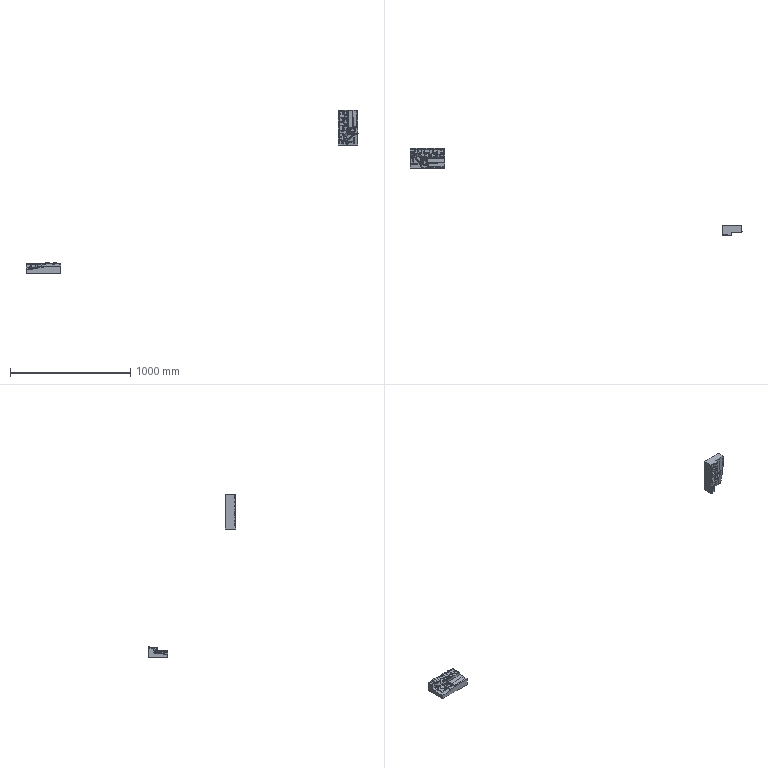NC program | NX | posted with a generic post | part box 2756 x 729.572 x 1353 mm
Lines 43585 to 44366 of 54396:
(ZLEVEL_PROFILE_3 , TOOL : D12)
N87150 M6
N87152 G54
N87154 G17 G0 G90 X-15.26 Y-84.156 B0. C0. S3000 M3
N87156 G43 Z97. H0
N87158 Z82.254
N87160 G94 G1 X-2.438 Y-83.975 Z81.918 F2500.
N87162 X0. Y-83.973 Z81.854
N87164 X-2.438 Y-83.975
N87166 X-31.79 Y-84.389
N87168 X-41.451 Y-84.428
N87170 X-43.147 Y-84.322
N87172 G2 X-50.227 Y-77.434 R7.65
N87174 G1 X-51.514 Y-77.439 Z81.655
N87176 G3 X-47.378 Y-83.482 R6.752
N87178 X-41.451 Y-84.694 R15.56
N87180 G1 X0. Y-84.333
N87182 Z84.655
N87184 G0 Z97.
N87186 X-76.288 Y-83.954
N87188 Z82.254
N87190 G1 X-72.831 Y-84.154 Z82.163
N87192 X-71.135 Y-84.11 Z82.119
N87194 X-70.497 Y-84.08 Z82.102
N87196 X-68.796 Y-83.61 Z82.056
N87198 X-67.273 Y-82.718 Z82.01
N87200 X-66.03 Y-81.466 Z81.964
N87202 X-65.15 Y-79.936 Z81.917
N87204 X-64.693 Y-78.231 Z81.871
N87206 X-64.668 Y-77.593 Z81.854
N87208 G2 X-71.135 Y-84.11 R6.785
N87210 G1 X-72.831 Y-84.154
N87212 X-83.009 Y-83.563
N87214 X-83.167 Y-83.542
N87216 X-87.688 Y-80.237
N87218 Z84.854
N87220 G0 Z97.
N87222 X-86.71 Y-84.276
N87224 Z82.054
N87226 G1 X-90.277 Y-84.161 Z81.961
N87228 X-95.479 Y-83.84 Z81.825
N87230 X-96.889 Y-83.466 Z81.786
N87232 X-98.189 Y-82.805 Z81.748
N87234 X-99.324 Y-81.888 Z81.71
N87236 X-100.241 Y-80.755 Z81.672
N87238 X-100.541 Y-80.183 Z81.655
N87240 G3 X-94.835 Y-83.88 R6.922
N87242 X-74.528 Y-84.537 R347.568
N87244 G1 X-73.463 Y-84.597
N87246 G3 X-68.845 Y-84.09 R14.083
N87248 X-63.737 Y-77.565 R7.018
N87250 G1 X-63.393 Y-77.56 Z81.555
N87252 X-63.108 Y-77.556 Z81.455
N87254 G2 X-66.891 Y-83.651 R7.004
N87256 X-71.649 Y-84.818 R10.426
N87258 X-104.334 Y-84.066 R619.573
N87260 X-111.303 Y-79.673 R8.39
N87262 G1 Z84.455
N87264 G0 Z97.
N87266 X-15.26 Y-84.692
N87268 Z81.855
N87270 G1 X-2.438 Y-84.565 Z81.519
N87272 X0. Y-84.592 Z81.455
N87274 X-2.438 Y-84.565
N87276 X-18.552 Y-84.725
N87278 X-22.793 Y-84.765
N87280 X-41.451 Y-84.881
N87282 G2 X-48.498 Y-83.558 R19.928
N87284 X-52.802 Y-77.444 R6.709
N87286 G1 X-54.089 Y-77.449 Z81.256
N87288 G3 X-49.43 Y-83.717 R6.783
N87290 X-41.451 Y-85.03 R26.196
N87292 G1 X-4.134 Y-84.771
N87294 X0.003 Y-84.763
N87296 Z84.256
N87298 G0 Z97.
N87300 X-73.803 Y-85.035
N87302 Z81.655
N87304 G1 X-71.983 Y-85.034 Z81.608
N87306 X-71.109 Y-85.039 Z81.585
N87308 X-69.38 Y-84.808 Z81.539
N87310 X-67.698 Y-84.345 Z81.493
N87312 X-66.895 Y-83.999 Z81.47
N87314 X-66.291 Y-83.731 Z81.453
N87316 X-64.897 Y-82.723 Z81.408
N87318 X-63.778 Y-81.416 Z81.363
N87320 X-62.997 Y-79.883 Z81.318
N87322 X-62.596 Y-78.21 Z81.273
N87324 X-62.579 Y-77.55 Z81.256
N87326 G2 X-66.895 Y-83.999 R7.261
N87328 X-71.983 Y-85.034 R12.732
N87330 X-109.155 Y-84.389 R1066.044
N87332 G1 X-115.237 Y-83.793
N87334 X-116.299 Y-83.542
N87336 X-116.933 Y-83.253
N87338 X-120.751 Y-78.147
N87340 Z84.256
N87342 G0 Z97.
N87344 X-115.867 Y-84.489
N87346 Z81.456
N87348 G1 X-119.405 Y-84.298 Z81.363
N87350 X-122.87 Y-83.978 Z81.272
N87352 X-123.501 Y-83.932 Z81.255
N87354 X-125.167 Y-83.42 Z81.21
N87356 X-126.644 Y-82.494 Z81.164
N87358 X-127.831 Y-81.217 Z81.118
N87360 X-128.646 Y-79.676 Z81.073
N87362 X-128.81 Y-79.066 Z81.056
N87364 G3 X-122.87 Y-83.978 R6.646
N87366 X-107.604 Y-84.805 R201.793
N87368 X-71.983 Y-85.161 R1612.787
N87370 G1 X-71.135 Y-85.134
N87372 G3 X-66.895 Y-84.243 R11.864
N87374 X-62.162 Y-77.545 R7.318
N87376 G1 Z84.056
N87378 G0 Z97.
N87380 X-15.258 Y-84.985
N87382 Z81.456
N87384 G1 X-5.828 Y-84.9 Z81.209
N87386 X0.003 Y-84.891 Z81.056
N87388 G3 X-11.659 Y-84.952 R1562.88
N87390 G2 X-41.451 Y-85.119 R4404.057
N87392 X-50.375 Y-83.867 R32.265
N87394 X-55.377 Y-77.455 R6.912
N87396 G1 X-56.665 Y-77.46 Z80.856
N87398 G3 X-53.377 Y-83.029 R6.44
N87400 X-49.749 Y-84.374 R12.414
N87402 X-41.309 Y-85.197 R41.905
N87404 G1 X-21.096 Y-85.111
N87406 G2 X0. Y-85.003 R1960.321
N87408 G1 Z83.856
N87410 G0 Z97.
N87412 X-72.868 Y-85.26
N87414 Z81.256
N87416 G1 X-71.135 Y-85.251 Z81.211
N87418 X-70.264 Y-85.238 Z81.188
N87420 X-68.524 Y-84.967 Z81.142
N87422 X-66.837 Y-84.458 Z81.096
N87424 X-66.047 Y-84.093 Z81.073
N87426 X-65.441 Y-83.811 Z81.055
N87428 X-64.055 Y-82.773 Z81.01
N87430 X-62.945 Y-81.444 Z80.965
N87432 X-62.171 Y-79.895 Z80.919
N87434 X-61.775 Y-78.21 Z80.874
N87436 X-61.758 Y-77.542 Z80.856
N87438 G2 X-66.047 Y-84.093 R7.435
N87440 X-71.135 Y-85.251 R12.626
N87442 X-117.782 Y-84.813 R1613.418
N87444 X-130.503 Y-83.973 R149.134
N87446 X-135.944 Y-80.062 R6.777
N87448 G1 X-136.372 Y-80.074 Z80.845
N87450 X-136.795 Y-80.083 Z80.833
N87452 X-137.219 Y-80.093 Z80.821
N87454 X-137.638 Y-80.1 Z80.809
N87456 X-138.035 Y-80.097 Z80.798
N87458 X-138.43 Y-80.093 Z80.786
N87460 X-138.826 Y-80.09 Z80.774
N87462 X-139.222 Y-80.086 Z80.762
N87464 X-139.618 Y-80.083 Z80.751
N87466 X-140.014 Y-80.08 Z80.739
N87468 X-140.409 Y-80.076 Z80.727
N87470 X-140.805 Y-80.073 Z80.715
N87472 X-141.2 Y-80.069 Z80.704
N87474 X-141.595 Y-80.065 Z80.692
N87476 X-141.991 Y-80.062 Z80.68
N87478 X-142.385 Y-80.058 Z80.669
N87480 X-142.779 Y-80.054 Z80.657
N87482 G3 X-137.418 Y-83.994 R6.767
N87484 X-125.542 Y-84.85 R124.376
N87486 X-71.135 Y-85.333 R1794.109
N87488 X-66.047 Y-84.307 R13.761
N87490 X-61.435 Y-77.539 R7.498
N87492 G1 Z83.657
N87494 G0 Z97.
N87496 X-15.255 Y-85.116
N87498 Z81.056
N87500 G1 X-14.786 Y-85.112 Z81.044
N87502 X0.006 Y-85.074 Z80.657
N87504 G3 X-29.578 Y-85.221 R6272.571
N87506 G1 X-41.451 Y-85.26
N87508 X-42.299 Y-85.272
N87510 G2 X-51.075 Y-84.389 R54.431
N87512 X-55.736 Y-82.252 R9.873
N87514 X-57.952 Y-77.465 R6.131
N87516 G1 X-59.24 Y-77.47 Z80.457
N87518 G3 X-57.002 Y-82.275 R6.156
N87520 X-52.529 Y-84.363 R9.858
N87522 X-42.235 Y-85.297 R55.422
N87524 G1 X-39.755 Y-85.29
N87526 X-16.856 Y-85.187
N87528 X-5.041 Y-85.125
N87530 G2 X-0.004 Y-85.131 R401.668
N87532 G1 Z83.457
N87534 G0 Z97.
N87536 X-72.13 Y-85.434
N87538 Z80.857
N87540 G1 X-72.02 Y-85.436 Z80.854
N87542 X-71.095 Y-85.41 Z80.83
N87544 X-69.439 Y-85.285 Z80.786
N87546 X-68.636 Y-85.227 Z80.765
N87548 X-67.248 Y-84.926 Z80.728
N87550 X-65.91 Y-84.445 Z80.691
N87552 X-65.198 Y-84.07 Z80.67
N87554 X-64.601 Y-83.767 Z80.652
N87556 X-63.276 Y-82.712 Z80.608
N87558 X-62.222 Y-81.387 Z80.563
N87560 X-61.492 Y-79.859 Z80.519
N87562 X-61.124 Y-78.207 Z80.475
N87564 X-61.113 Y-77.537 Z80.457
N87566 G2 X-65.198 Y-84.07 R7.468
N87568 X-69.439 Y-85.285 R10.776
N87570 X-73.68 Y-85.407 R45.93
N87572 G1 X-74.528 Y-85.392
N87574 G2 X-117.782 Y-85.229 R2539.324
N87576 X-142.923 Y-84.276 R450.056
N87578 X-149.269 Y-80.042 R7.642
N87580 G1 X-149.678 Y-80.041 Z80.444
N87582 X-150.085 Y-80.038 Z80.431
N87584 X-150.492 Y-80.036 Z80.417
N87586 X-150.899 Y-80.034 Z80.404
N87588 X-151.306 Y-80.032 Z80.391
N87590 X-151.713 Y-80.029 Z80.377
N87592 X-152.12 Y-80.027 Z80.364
N87594 X-152.528 Y-80.026 Z80.351
N87596 X-152.933 Y-80.023 Z80.337
N87598 X-153.34 Y-80.02 Z80.324
N87600 X-153.747 Y-80.018 Z80.311
N87602 X-154.154 Y-80.016 Z80.297
N87604 X-154.561 Y-80.014 Z80.284
N87606 X-154.968 Y-80.011 Z80.271
N87608 X-155.375 Y-80.009 Z80.258
N87610 G3 X-150.241 Y-84.012 R6.619
N87612 G1 X-149.162 Y-84.173
N87614 X-141.529 Y-84.814
N87616 G3 X-111.845 Y-85.42 R967.084
N87618 X-71.135 Y-85.414 R4122.292
N87620 G1 X-70.287 Y-85.401
N87622 G3 X-66.047 Y-84.618 R12.922
N87624 X-60.811 Y-77.534 R7.695
N87626 G1 Z83.258
N87628 G0 Z97.
N87630 X-15.266 Y-85.208
N87632 Z80.657
N87634 G1 X-3.286 Y-85.153 Z80.343
N87636 X-0.005 Y-85.158 Z80.258
N87638 X-3.286 Y-85.153
N87640 X-16.856 Y-85.215
N87642 X-42.299 Y-85.323
N87644 G2 X-51.295 Y-84.803 R74.498
N87646 X-56.208 Y-83.598 R20.754
N87648 X-60.527 Y-77.476 R6.696
N87650 G1 Z83.258
N87652 G0 Z97.
N87654 X-147.529 Y-84.844
N87656 Z80.458
N87658 G1 X-148.314 Y-84.813 Z80.437
N87660 X-150.016 Y-84.761 Z80.392
N87662 X-154.043 Y-84.328 Z80.286
N87664 X-156.381 Y-83.891 Z80.224
N87666 X-158.123 Y-83.159 Z80.175
N87668 X-159.631 Y-82.02 Z80.125
N87670 X-160.812 Y-80.545 Z80.076
N87672 X-161.112 Y-79.941 Z80.058
N87674 G3 X-155.717 Y-84.015 R7.578
N87676 X-148.314 Y-84.813 R48.317
N87678 X-121.174 Y-85.447 R801.832
N87680 X-70.287 Y-85.428 R4192.566
N87682 X-66.047 Y-84.761 R13.62
N87684 X-61.107 Y-80.35 R8.22
N87686 X-57.081 Y-83.781 R7.132
N87688 X-52.477 Y-84.819 R22.701
N87690 X-43.996 Y-85.33 R75.99
N87692 G1 X-4.982 Y-85.166
N87694 X0.001 Y-85.165
N87696 Z79.858
N87698 X-4.982 Y-85.166
N87700 X-44.844 Y-85.333
N87702 X-46.656 Y-85.317
N87704 G2 X-56.513 Y-84.355 R55.858
N87706 X-61.527 Y-81.644 R9.356
N87708 X-66.048 Y-84.871 R8.866
N87710 X-69.704 Y-85.437 R12.577
N87712 X-112.693 Y-85.549 R6359.498
N87714 X-143.225 Y-85.246 R1397.155
N87716 G1 X-143.737 Y-85.236
N87718 X-151.706 Y-84.939
N87720 X-152.554 Y-84.891
N87722 G2 X-162.732 Y-82.614 R30.47
N87724 X-167.024 Y-78.15 R7.436
N87726 G1 X-167.392 Y-77.962 Z79.847
N87728 X-167.746 Y-77.768 Z79.835
N87730 X-168.1 Y-77.575 Z79.823
N87732 X-168.454 Y-77.381 Z79.811
N87734 X-168.781 Y-77.18 Z79.8
N87736 X-169.124 Y-76.983 Z79.788
N87738 X-169.513 Y-76.799 Z79.776
N87740 X-169.864 Y-76.604 Z79.764
N87742 X-170.215 Y-76.41 Z79.753
N87744 X-170.564 Y-76.215 Z79.741
N87746 X-170.917 Y-76.02 Z79.729
N87748 X-171.259 Y-75.824 Z79.717
N87750 X-171.59 Y-75.625 Z79.706
N87752 X-171.954 Y-75.433 Z79.694
N87754 X-172.298 Y-75.237 Z79.682
N87756 X-172.641 Y-75.041 Z79.67
N87758 X-172.981 Y-74.845 Z79.659
N87760 G3 X-168.85 Y-80.672 R8.016
N87762 X-151.706 Y-85.203 R38.229
N87764 X-126.6 Y-85.575 R1114.804
N87766 X-103.563 Y-85.571 R3081.8
N87768 G1 X-69.439 Y-85.437
N87770 G3 X-66.895 Y-85.164 R12.488
N87772 X-61.928 Y-82.512 R9.408
N87774 X-56.945 Y-84.53 R12.152
N87776 X-46.54 Y-85.34 R62.082
N87778 G1 X-4.982 Y-85.166
N87780 X0.001 Y-85.165
N87782 Z79.459
N87784 X-4.982 Y-85.166
N87786 X-48.236 Y-85.34
N87788 G2 X-58.362 Y-84.501 R58.672
N87790 X-62.256 Y-83.125 R12.186
N87792 X-68.591 Y-85.419 R10.432
N87794 G1 X-69.439 Y-85.437
N87796 X-114.389 Y-85.626
N87798 X-126.067 Y-85.621
N87800 G2 X-151.818 Y-85.37 R1382.193
N87802 X-175.375 Y-77.615 R42.102
N87804 X-178.764 Y-72.06 R8.26
N87806 G1 X-179.116 Y-71.85 Z79.447
N87808 X-179.459 Y-71.639 Z79.436
N87810 X-179.803 Y-71.428 Z79.424
N87812 X-180.146 Y-71.217 Z79.412
N87814 X-180.49 Y-71.006 Z79.4
N87816 X-180.833 Y-70.795 Z79.389
N87818 X-181.177 Y-70.584 Z79.377
N87820 X-181.521 Y-70.373 Z79.365
N87822 X-181.864 Y-70.162 Z79.353
N87824 X-182.208 Y-69.951 Z79.342
N87826 X-182.551 Y-69.74 Z79.33
N87828 X-182.895 Y-69.529 Z79.318
N87830 X-183.239 Y-69.318 Z79.306
N87832 X-183.582 Y-69.107 Z79.295
N87834 X-183.926 Y-68.896 Z79.283
N87836 X-184.269 Y-68.686 Z79.271
N87838 X-184.605 Y-68.47 Z79.259
N87840 X-182.089 Y-73.381
N87842 X-181.39 Y-74.122
N87844 G3 X-151.706 Y-85.521 R46.715
N87846 X-117.782 Y-85.642 R2121.63
N87848 G1 X-68.591 Y-85.432
N87850 G3 X-62.558 Y-83.66 R11.672
N87852 X-58.694 Y-84.674 R18.227
N87854 X-49.084 Y-85.35 R62.914
N87856 G1 X-4.982 Y-85.166
N87858 X0.001 Y-85.165
N87860 Z79.06
N87862 X-4.982 Y-85.166
N87864 X-49.932 Y-85.355
N87866 G2 X-59.262 Y-84.799 R69.021
N87868 X-62.788 Y-84.029 R20.683
N87870 X-68.591 Y-85.432 R12.548
N87872 G1 X-124.159 Y-85.669
N87874 G2 X-151.229 Y-85.628 R2342.368
N87876 X-161.035 Y-84.597 R50.724
N87878 X-188.175 Y-68.956 R52.233
N87880 G1 X-188.736 Y-68.3
N87882 X-190.408 Y-64.913
N87884 X-190.506 Y-64.151
N87886 X-190.84 Y-63.908 Z79.049
N87888 X-191.168 Y-63.665 Z79.038
N87890 X-191.496 Y-63.422 Z79.027
N87892 X-191.825 Y-63.178 Z79.015
N87894 X-192.153 Y-62.935 Z79.004
N87896 X-192.481 Y-62.692 Z78.993
N87898 X-192.809 Y-62.448 Z78.982
N87900 X-193.137 Y-62.205 Z78.971
N87902 X-193.465 Y-61.962 Z78.96
N87904 X-193.794 Y-61.718 Z78.949
N87906 X-194.122 Y-61.475 Z78.938
N87908 X-194.45 Y-61.231 Z78.927
N87910 X-194.778 Y-60.988 Z78.916
N87912 X-195.106 Y-60.745 Z78.905
N87914 X-195.434 Y-60.501 Z78.893
N87916 X-195.763 Y-60.258 Z78.882
N87918 X-196.091 Y-60.014 Z78.871
N87920 X-196.418 Y-59.771 Z78.86
N87922 G3 X-193.297 Y-65.246 R14.336
N87924 X-175.751 Y-79.308 R72.566
N87926 X-151.706 Y-85.699 R50.267
N87928 G1 X-133.896 Y-85.71
N87930 X-67.743 Y-85.421
N87932 G3 X-62.972 Y-84.359 R14.903
N87934 X-58.414 Y-85.053 R39.933
N87936 X-51.629 Y-85.361 R77.462
N87938 G1 X-4.982 Y-85.166
N87940 X0.001 Y-85.165
N87942 Z78.661
N87944 X-4.982 Y-85.166
N87946 X-53.13 Y-85.367
N87948 G2 X-63.037 Y-84.62 R62.606
N87950 G1 X-65.111 Y-85.11
N87952 G2 X-67.816 Y-85.431 R11.986
N87954 G1 X-143.225 Y-85.748
N87956 X-152.554 Y-85.725
N87958 X-154.251 Y-85.681
N87960 G2 X-176.616 Y-79.18 R51.501
N87962 X-189.023 Y-70.199 R66.39
N87964 X-200.313 Y-59.833 R117.66
N87966 G1 X-200.897 Y-59.055
N87968 X-202.324 Y-55.39
N87970 Z81.661
N87972 G0 Z97.
N87974 X-233.773 Y-47.613
N87976 Z81.056
N87978 G1 X-231.945 Y-47.26 Z81.008
N87980 X-230.581 Y-46.874 Z80.971
N87982 X-230.021 Y-46.662 Z80.955
N87984 X-228.743 Y-45.803 Z80.915
N87986 X-227.726 Y-44.645 Z80.874
N87988 X-227.038 Y-43.266 Z80.834
N87990 X-226.726 Y-41.758 Z80.793
N87992 X-226.808 Y-40.219 Z80.753
N87994 X-227.281 Y-38.753 Z80.713
N87996 X-228.113 Y-37.456 Z80.672
N87998 X-228.542 Y-37.039 Z80.657
N88000 G2 X-230.581 Y-46.874 R5.954
N88002 X-241.798 Y-48.07 R33.455
N88004 X-248.063 Y-40.695 R6.722
N88006 G1 X-248.442 Y-40.848 Z80.557
N88008 X-248.709 Y-41.008 Z80.457
N88010 G3 X-240.598 Y-48.951 R7.685
N88012 G2 X-223.856 Y-48.894 R159.009
N88014 G3 X-216.714 Y-43.031 R6.877
N88016 G1 X-216.347 Y-43.263 Z80.357
N88018 X-216.115 Y-43.472 Z80.258
N88020 G2 X-224.644 Y-49.614 R7.705
N88022 G1 X-225.492 Y-49.503
N88024 G3 X-240.758 Y-49.42 R118.273
N88026 G2 X-249.122 Y-41.068 R8.095
N88028 G1 X-249.3 Y-41.087 Z80.158
N88030 X-249.443 Y-41.102 Z80.058
N88032 G3 X-240.758 Y-49.793 R8.457
N88034 G1 X-232.277 Y-49.686
N88036 G2 X-224.644 Y-50.093 R55.651
N88038 G3 X-215.718 Y-43.609 R8.158
N88040 G1 X-215.556 Y-43.673 Z79.958
N88042 X-215.406 Y-43.732 Z79.858
N88044 G2 X-224.759 Y-50.443 R8.507
N88046 G3 X-232.277 Y-50.025 R57.669
N88048 G1 X-240.758 Y-50.114
N88050 G2 X-249.53 Y-42.898 R8.639
N88052 X-249.719 Y-41.125 R6.395
N88054 G1 X-249.836 Y-41.137 Z79.758
N88056 X-249.942 Y-41.148 Z79.659
N88058 G3 X-240.758 Y-50.368 R9.012
N88060 G1 X-232.277 Y-50.309
N88062 G2 X-224.85 Y-50.74 R55.695
N88064 G3 X-215.139 Y-43.751 R8.789
N88066 G1 X-215.024 Y-43.396 Z79.619
N88068 X-214.925 Y-43.036 Z79.579
N88070 X-214.833 Y-42.674 Z79.539
N88072 X-214.765 Y-42.31 Z79.499
N88074 X-214.719 Y-41.949 Z79.459
N88076 G2 X-224.974 Y-51.001 R9.063
N88078 G3 X-232.277 Y-50.564 R50.782
N88080 G1 X-240.758 Y-50.601
N88082 X-241.05 Y-50.597
N88084 G2 X-250.163 Y-41.182 R9.24
N88086 G1 X-250.272 Y-41.205 Z79.359
N88088 X-250.404 Y-41.232 Z79.259
N88090 G3 X-241.05 Y-50.799 R9.492
N88092 G1 X-240.758 Y-50.803
N88094 X-233.125 Y-50.769
N88096 G2 X-224.644 Y-51.255 R61.029
N88098 G3 X-217.859 Y-49.145 R9.075
N88100 X-214.493 Y-41.659 R8.833
N88102 G1 X-214.354 Y-41.666 Z79.16
N88104 X-214.211 Y-41.674 Z79.06
N88106 G2 X-216.736 Y-48.439 R8.621
N88108 G1 X-216.961 Y-48.662
N88110 G2 X-225.215 Y-51.412 R9.802
N88112 G3 X-230.581 Y-50.99 R44.959
N88114 G1 X-232.277 Y-50.965
N88116 X-240.758 Y-50.991
N88118 G2 X-247.543 Y-48.31 R9.389
N88120 X-250.661 Y-41.28 R9.289
N88122 G1 X-250.781 Y-41.303 Z78.96
N88124 X-250.922 Y-41.329 Z78.86
N88126 G3 X-247.543 Y-48.558 R9.162
N88128 X-241.182 Y-51.137 R9.711
N88130 G1 X-240.758 Y-51.148
N88132 X-233.125 Y-51.13
N88134 G2 X-225.009 Y-51.593 R62.326
N88136 G3 X-217.648 Y-49.57 R10.025
N88138 G1 X-217.011 Y-49.077
N88140 G3 X-213.915 Y-41.714 R8.498
N88142 G1 X-213.591 Y-41.769 Z78.661
N88144 G2 X-218.721 Y-50.519 R8.717
N88146 X-224.644 Y-51.811 R10.732
N88148 G3 X-230.648 Y-51.329 R52.182
N88150 G1 X-232.277 Y-51.293
N88152 X-240.758 Y-51.304
N88154 G2 X-246.695 Y-49.431 R9.989
N88156 X-250.718 Y-44.591 R10.694
N88158 X-251.278 Y-41.363 R9.119
N88160 G1 X-251.431 Y-41.377 Z78.561
N88162 X-251.639 Y-41.396 Z78.461
N88164 G3 X-250.717 Y-45.438 R7.355
N88166 X-245.847 Y-50.118 R11.606
N88168 X-240.758 Y-51.432 R9.828
N88170 G1 X-232.277 Y-51.43
N88172 G2 X-225.062 Y-51.912 R53.301
N88174 G3 X-222.1 Y-51.845 R9.484
N88176 X-216.748 Y-49.672 R14.075
N88178 X-213.148 Y-42.045 R8.006
N88180 G1 Z81.461
N88182 G0 Z97.
N88184 X-15.26 Y-85.209
N88186 Z78.861
N88188 G1 X-4.982 Y-85.166 Z78.591
N88190 X0.001 Y-85.165 Z78.461
N88192 X-4.982 Y-85.166
N88194 X-54.173 Y-85.371
N88196 G2 X-62.46 Y-84.908 R73.364
N88198 G3 X-64.222 Y-85.015 R5.123
N88200 G2 X-67.743 Y-85.431 R15.252
N88202 G1 X-150.858 Y-85.769
N88204 X-151.706 Y-85.768
N88206 G2 X-174.605 Y-80.489 R51.652
N88208 G1 X-175.284 Y-80.155
N88210 X-175.517 Y-80.035
N88212 G2 X-187.983 Y-71.584 R62.585
N88214 G1 X-188.175 Y-71.417
N88216 G2 X-205.357 Y-56.446 R245.794
N88218 G1 X-205.986 Y-55.682
N88220 X-208.226 Y-51.17
N88222 Z81.461
N88224 G0 Z97.
N88226 X-242.31 Y-51.451
N88228 Z78.661
N88230 G1 X-243.448 Y-51.258 Z78.631
N88232 X-244.992 Y-50.732 Z78.588
N88234 X-247.044 Y-49.647 Z78.527
N88236 X-248.506 Y-48.596 Z78.48
N88238 X-249.808 Y-47.351 Z78.433
N88240 X-250.355 Y-46.661 Z78.41
N88242 X-250.789 Y-46.113 Z78.392
N88244 X-251.468 Y-44.861 Z78.354
N88246 X-251.919 Y-43.51 Z78.317
N88248 X-252.128 Y-42.1 Z78.28
N88250 X-252.11 Y-41.402 Z78.261
N88252 G3 X-250.355 Y-46.661 R8.128
N88254 X-246.266 Y-50.059 R12.914
N88256 G1 X-245.681 Y-50.368
N88258 G3 X-241.06 Y-51.538 R10.115
N88260 X-233.973 Y-51.567 R563.268
N88262 G2 X-225.951 Y-51.925 R56.038
N88264 G1 X-224.644 Y-52.078
N88266 G3 X-218.707 Y-51.041 R13.142
N88268 X-214.098 Y-47.799 R10.447
N88270 G1 X-214.089 Y-47.942
N88272 G3 X-211.608 Y-52.454 R7.121
N88274 X-186.836 Y-72.94 R2260.884
N88276 X-178.138 Y-78.891 R62.846
N88278 G1 X-177.998 Y-78.97
N88280 G3 X-151.706 Y-85.785 R52.568
N88282 G1 X-150.858 Y-85.781
N88284 X-67.743 Y-85.431
N88286 G3 X-64.784 Y-85.236 R23.658
N88288 G1 X-64.345 Y-85.15
N88290 G2 X-62.429 Y-85.055 R6.755
N88292 G3 X-55.021 Y-85.374 R74.217
N88294 G1 X-4.982 Y-85.166
N88296 X0.001 Y-85.165
N88298 Z78.062
N88300 X-4.982 Y-85.166
N88302 X-55.965 Y-85.378
N88304 G2 X-61.564 Y-85.236 R94.764
N88306 G1 X-62.739 Y-85.139
N88308 G3 X-63.502 Y-85.157 R3.65
N88310 G2 X-67.743 Y-85.431 R33.517
N88312 G1 X-151.706 Y-85.785
N88314 G2 X-177.993 Y-79.208 R52.919
N88316 X-186.553 Y-73.497 R61.156
N88318 X-205.986 Y-57.714 R1297.704
N88320 G1 X-207.752 Y-56.446
N88322 X-216.83 Y-50.589
N88324 G2 X-223.003 Y-52.212 R19.814
N88326 X-224.875 Y-52.181 R8.382
N88328 G1 X-225.015 Y-52.163
N88330 G3 X-232.733 Y-51.661 R60.779
N88332 G1 X-241.05 Y-51.65
N88334 G2 X-244.242 Y-51.09 R9.433
N88336 G1 X-244.707 Y-50.922
N88338 G2 X-251.001 Y-46.461 R14.457
N88340 X-252.667 Y-41.376 R7.445
N88342 G1 Z81.062
N88344 G0 Z97.
N88346 X-273.184 Y-42.947
N88348 Z78.461
N88350 G1 X-269.594 Y-42.514 Z78.367
N88352 X-267.898 Y-41.348 Z78.313
N88354 X-267.468 Y-40.931 Z78.297
N88356 X-266.576 Y-39.51 Z78.253
N88358 X-266.113 Y-37.898 Z78.209
N88360 X-266.114 Y-36.22 Z78.165
N88362 X-266.581 Y-34.608 Z78.121
N88364 X-267.476 Y-33.189 Z78.077
N88366 X-267.907 Y-32.774 Z78.062
N88368 G2 X-267.898 Y-41.348 R5.964
N88370 G1 X-269.594 Y-42.514
N88372 X-279.797 Y-43.745
N88374 X-285.708 Y-43.915
N88376 X-286.394 Y-43.901
N88378 X-286.445 Y-44.234 Z77.962
N88380 X-286.49 Y-44.528 Z77.862
N88382 X-285.708 Y-44.534
N88384 X-267.05 Y-44.41
N88386 X-260.522 Y-44.231
N88388 G2 X-251.923 Y-46.285 R17.077
N88390 G3 X-244.151 Y-51.233 R17.981
N88392 X-240.758 Y-51.76 R10.901
N88394 G1 X-233.125 Y-51.773
N88396 G2 X-224.644 Y-52.312 R63.578
N88398 G3 X-217.932 Y-51.381 R20.108
N88400 G2 X-204.471 Y-59.471 R57.807
N88402 G3 X-186.479 Y-73.845 R3373.774
N88404 X-168.054 Y-83.542 R55.968
N88406 X-152.554 Y-85.786 R53.916
N88408 G1 X-66.047 Y-85.412
N88410 G2 X-61.866 Y-85.286 R25.961
N88412 G3 X-57.494 Y-85.387 R80.214
N88414 G1 X-4.982 Y-85.166
N88416 X0.001 Y-85.165
N88418 Z77.662
N88420 X-4.982 Y-85.166
N88422 X-59.262 Y-85.393
N88424 G3 X-66.047 Y-85.421 R75.196
N88426 G1 X-153.402 Y-85.779
N88428 G2 X-172.061 Y-82.285 R54.369
N88430 X-186.329 Y-74.208 R55.865
N88432 G1 X-189.023 Y-72.107
N88434 X-204.289 Y-59.985
N88436 G3 X-218.466 Y-51.839 R49.793
N88438 G2 X-224.644 Y-52.413 R27.324
N88440 G3 X-233.125 Y-51.862 R60.255
N88442 G1 X-240.758 Y-51.843
N88444 X-241.606 Y-51.818
N88446 G2 X-246.695 Y-50.39 R15.467
N88448 X-250.498 Y-48.322 R48.18
N88450 X-255.897 Y-46.163 R24.284
N88452 G3 X-260.577 Y-45.004 R9.46
N88454 G1 X-265.354 Y-45.076
N88456 X-286.55 Y-44.968
N88458 X-286.563 Y-45.148 Z77.563
N88460 X-286.575 Y-45.309 Z77.463
N88462 X-262.809 Y-45.534
N88464 X-260.512
N88466 G2 X-256.044 Y-46.701 R9.142
N88468 G3 X-250.088 Y-49.029 R23.234
N88470 X-245.847 Y-50.889 R47.625
N88472 X-240.758 Y-51.916 R14.318
N88474 G1 X-233.125 Y-51.946
N88476 X-231.826 Y-51.957
N88478 G2 X-225.631 Y-52.38 R51.767
N88480 G1 X-225.492 Y-52.398
N88482 G3 X-222.1 Y-52.476 R17.334
N88484 G1 X-218.814 Y-52.195
N88486 G2 X-204.565 Y-60.097 R48.825
N88488 G1 X-203.441 Y-60.995
N88490 X-187.327 Y-73.657
N88492 X-186.605 Y-74.228
N88494 G3 X-167.82 Y-83.771 R54.458
N88496 X-152.554 Y-85.786 R57.055
N88498 G1 X-65.198 Y-85.417
N88500 G2 X-63.182 Y-85.379 R41.494
N88502 G1 X-60.11 Y-85.396
N88504 X-4.982 Y-85.166
N88506 X0.001 Y-85.165
N88508 X0. Z77.263
N88510 X-4.982 Y-85.166
N88512 X-66.895 Y-85.424
N88514 X-71.135 Y-85.446
N88516 X-153.402 Y-85.783
N88518 G2 X-172.061 Y-82.493 R56.938
N88520 X-180.307 Y-78.645 R58.624
N88522 X-185.663 Y-75.138 R48.942
N88524 G1 X-186.873 Y-74.228
N88526 X-204.908 Y-60.12
N88528 G3 X-219.069 Y-52.493 R47.62
N88530 G1 X-222.417 Y-52.605
N88532 G2 X-224.644 Y-52.564 R21.529
N88534 G3 X-232.341 Y-52.021 R57.877
N88536 G1 X-240.758 Y-51.99
N88538 X-241.606 Y-51.957
N88540 G2 X-247.543 Y-50.422 R20.635
N88542 G3 X-251.152 Y-49.18 R29.651
N88544 G2 X-256.353 Y-47.029 R22.528
N88546 G3 X-260.519 Y-45.903 R8.602
N88548 G1 X-262.809 Y-45.879
N88550 X-286.59 Y-45.596
N88552 X-286.597 Y-45.734 Z77.163
N88554 X-286.603 Y-45.855 Z77.064
N88556 X-284.012 Y-45.892
N88558 X-260.265 Y-46.274
N88560 G2 X-256.688 Y-47.24 R7.33
N88562 G3 X-251.14 Y-49.545 R24.056
N88564 G1 X-250.936 Y-49.602
N88566 X-246.695 Y-50.905
N88568 X-245.847 Y-51.183
N88570 G3 X-241.606 Y-52.017 R19.569
N88572 G1 X-240.758 Y-52.037
N88574 X-232.427 Y-52.072
N88576 G2 X-224.644 Y-52.638 R57.065
N88578 G3 X-219.969 Y-52.7 R54.15
N88580 G2 X-218.75 Y-52.903 R3.182
N88582 G1 X-218.338 Y-53.059
N88584 G2 X-204.525 Y-60.68 R46.998
N88586 G1 X-203.441 Y-61.537
N88588 X-187.104 Y-74.228
N88590 X-186.001 Y-75.074
N88592 G3 X-169.044 Y-83.542 R53.718
N88594 X-152.554 Y-85.786 R59.171
N88596 G1 X-71.135 Y-85.446
N88598 X-4.982 Y-85.166
N88600 X0. Y-85.165
N88602 Z76.864
N88604 X-4.982 Y-85.166
N88606 X-71.135 Y-85.446
N88608 X-153.402 Y-85.787
N88610 G2 X-171.213 Y-82.919 R58.495
N88612 X-186.209 Y-75.074 R52.71
N88614 G1 X-187.33 Y-74.228
N88616 X-205.137 Y-60.426
N88618 G3 X-219.143 Y-53.051 R46.855
N88620 X-220.102 Y-52.893 R3.215
N88622 G2 X-224.644 Y-52.7 R72.819
N88624 G3 X-232.397 Y-52.124 R56.473
N88626 G1 X-240.758 Y-52.08
N88628 X-240.853 Y-52.078
N88630 G2 X-246.181 Y-51.228 R19.736
N88632 G1 X-246.695 Y-51.071
N88634 X-251.086 Y-49.865
N88636 G2 X-256.759 Y-47.518 R24.762
N88638 G3 X-260.376 Y-46.528 R7.593
N88640 G1 X-286.611 Y-46.067
N88642 X-286.616 Y-46.183 Z76.764
N88644 X-286.62 Y-46.278 Z76.664
N88646 X-260.265 Y-46.773
N88648 G2 X-256.907 Y-47.712 R7.067
N88650 G3 X-251.784 Y-49.92 R24.316
N88652 G1 X-245.968 Y-51.426
N88654 G3 X-240.904 Y-52.12 R21.853
N88656 G1 X-240.758 Y-52.123
N88658 X-232.059 Y-52.178
N88660 G2 X-225.849 Y-52.603 R50.18
N88662 G1 X-224.644 Y-52.761
N88664 G3 X-221.252 Y-53.008 R61.985
N88666 G1 X-219.555 Y-53.17
N88668 G2 X-205.137 Y-60.633 R45.817
N88670 G1 X-203.441 Y-61.952
N88672 X-188.619 Y-73.381
N88674 X-187.511 Y-74.228
N88676 X-187.327 Y-74.363
N88678 X-186.408 Y-75.074
N88680 G3 X-169.517 Y-83.491 R52.255
N88682 X-153.402 Y-85.788 R58.795
N88684 G1 X-71.135 Y-85.446
N88686 X-4.982 Y-85.166
N88688 X0. Y-85.165
N88690 Z76.465
N88692 X-4.982 Y-85.166
N88694 X-71.135 Y-85.446
N88696 X-153.402 Y-85.788
N88698 G2 X-171.213 Y-83.021 R58.666
N88700 X-185.421 Y-75.921 R52.079
N88702 G1 X-186.579 Y-75.074
N88704 X-187.327 Y-74.496
N88706 X-187.691 Y-74.228